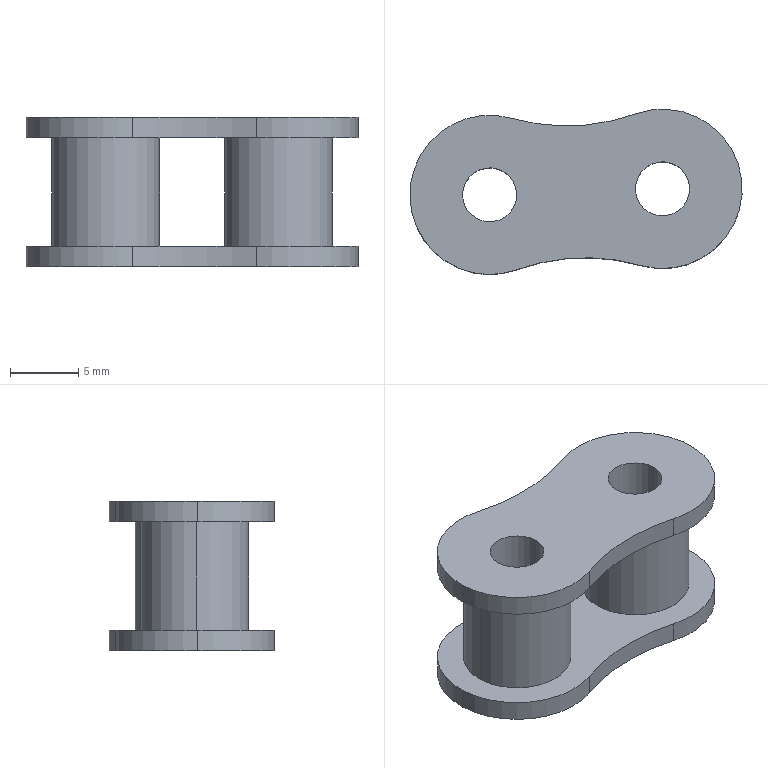Part | STEP file | CHES40-46-Part-17 | 1 solid | 22 faces | box 24.392 x 12.143 x 10.95 mm | volume 1237 mm3 | cylinder 18 | plane 4 | commonest cylinder face diameters 11.7 x6 3.97 x4 7.92 x4 29.64 x4
STEP:
#1=CARTESIAN_POINT('',(-99.678,72.735,-5.475));
#2=VERTEX_POINT('',#1);
#3=CARTESIAN_POINT('',(-103.646,72.597,-5.475));
#4=VERTEX_POINT('',#3);
#5=CARTESIAN_POINT('',(-101.662,72.666,-5.475));
#6=DIRECTION('',(0.,0.,1.));
#7=DIRECTION('',(-0.9994,-0.0349,0.));
#8=AXIS2_PLACEMENT_3D('',#5,#6,#7);
#9=CIRCLE('',#8,1.985);
#10=EDGE_CURVE('',#2,#4,#9,.T.);
#11=ORIENTED_EDGE('',*,*,#10,.F.);
#12=CARTESIAN_POINT('',(-99.678,72.735,5.475));
#13=VERTEX_POINT('',#12);
#14=CARTESIAN_POINT('',(-99.678,72.735,-5.475));
#15=DIRECTION('',(0.,0.,1.));
#16=VECTOR('',#15,1000.);
#17=LINE('',#14,#16);
#18=EDGE_CURVE('',#2,#13,#17,.T.);
#19=ORIENTED_EDGE('',*,*,#18,.T.);
#20=CARTESIAN_POINT('',(-103.646,72.597,5.475));
#21=VERTEX_POINT('',#20);
#22=CARTESIAN_POINT('',(-101.662,72.666,5.475));
#23=DIRECTION('',(0.,0.,1.));
#24=DIRECTION('',(-0.9994,-0.0349,0.));
#25=AXIS2_PLACEMENT_3D('',#22,#23,#24);
#26=CIRCLE('',#25,1.985);
#27=EDGE_CURVE('',#13,#21,#26,.T.);
#28=ORIENTED_EDGE('',*,*,#27,.T.);
#29=CARTESIAN_POINT('',(-103.646,72.597,-5.475));
#30=DIRECTION('',(0.,0.,1.));
#31=VECTOR('',#30,1000.);
#32=LINE('',#29,#31);
#33=EDGE_CURVE('',#4,#21,#32,.T.);
#34=ORIENTED_EDGE('',*,*,#33,.F.);
#35=EDGE_LOOP('',(#11,#19,#28,#34));
#36=FACE_OUTER_BOUND('',#35,.T.);
#37=CARTESIAN_POINT('',(-101.662,72.666,-5.475));
#38=DIRECTION('',(0.,0.,1.));
#39=DIRECTION('',(-0.9994,-0.0349,0.));
#40=AXIS2_PLACEMENT_3D('',#37,#38,#39);
#41=CYLINDRICAL_SURFACE('',#40,1.985);
#42=ADVANCED_FACE('',(#36),#41,.F.);
#43=CARTESIAN_POINT('',(-112.37,72.292,-5.475));
#44=VERTEX_POINT('',#43);
#45=CARTESIAN_POINT('',(-116.338,72.153,-5.475));
#46=VERTEX_POINT('',#45);
#47=CARTESIAN_POINT('',(-114.354,72.223,-5.475));
#48=DIRECTION('',(0.,0.,1.));
#49=DIRECTION('',(-0.9994,-0.0349,0.));
#50=AXIS2_PLACEMENT_3D('',#47,#48,#49);
#51=CIRCLE('',#50,1.985);
#52=EDGE_CURVE('',#44,#46,#51,.T.);
#53=ORIENTED_EDGE('',*,*,#52,.F.);
#54=CARTESIAN_POINT('',(-112.37,72.292,5.475));
#55=VERTEX_POINT('',#54);
#56=CARTESIAN_POINT('',(-112.37,72.292,-5.475));
#57=DIRECTION('',(0.,0.,1.));
#58=VECTOR('',#57,1000.);
#59=LINE('',#56,#58);
#60=EDGE_CURVE('',#44,#55,#59,.T.);
#61=ORIENTED_EDGE('',*,*,#60,.T.);
#62=CARTESIAN_POINT('',(-116.338,72.153,5.475));
#63=VERTEX_POINT('',#62);
#64=CARTESIAN_POINT('',(-114.354,72.223,5.475));
#65=DIRECTION('',(0.,0.,1.));
#66=DIRECTION('',(-0.9994,-0.0349,0.));
#67=AXIS2_PLACEMENT_3D('',#64,#65,#66);
#68=CIRCLE('',#67,1.985);
#69=EDGE_CURVE('',#55,#63,#68,.T.);
#70=ORIENTED_EDGE('',*,*,#69,.T.);
#71=CARTESIAN_POINT('',(-116.338,72.153,-5.475));
#72=DIRECTION('',(0.,0.,1.));
#73=VECTOR('',#72,1000.);
#74=LINE('',#71,#73);
#75=EDGE_CURVE('',#46,#63,#74,.T.);
#76=ORIENTED_EDGE('',*,*,#75,.F.);
#77=EDGE_LOOP('',(#53,#61,#70,#76));
#78=FACE_OUTER_BOUND('',#77,.T.);
#79=CARTESIAN_POINT('',(-114.354,72.223,-5.475));
#80=DIRECTION('',(0.,0.,1.));
#81=DIRECTION('',(-0.9994,-0.0349,0.));
#82=AXIS2_PLACEMENT_3D('',#79,#80,#81);
#83=CYLINDRICAL_SURFACE('',#82,1.985);
#84=ADVANCED_FACE('',(#78),#83,.F.);
#85=CARTESIAN_POINT('',(-120.201,72.018,-5.475));
#86=VERTEX_POINT('',#85);
#87=CARTESIAN_POINT('',(-112.752,77.849,-5.475));
#88=VERTEX_POINT('',#87);
#89=CARTESIAN_POINT('',(-114.354,72.223,-5.475));
#90=DIRECTION('',(0.,0.,-1.));
#91=DIRECTION('',(0.9994,0.0349,0.));
#92=AXIS2_PLACEMENT_3D('',#89,#90,#91);
#93=CIRCLE('',#92,5.85);
#94=EDGE_CURVE('',#86,#88,#93,.T.);
#95=ORIENTED_EDGE('',*,*,#94,.F.);
#96=CARTESIAN_POINT('',(-120.201,72.018,-3.975));
#97=VERTEX_POINT('',#96);
#98=CARTESIAN_POINT('',(-120.201,72.018,-5.475));
#99=DIRECTION('',(0.,0.,1.));
#100=VECTOR('',#99,1000.);
#101=LINE('',#98,#100);
#102=EDGE_CURVE('',#86,#97,#101,.T.);
#103=ORIENTED_EDGE('',*,*,#102,.T.);
#104=CARTESIAN_POINT('',(-112.752,77.849,-3.975));
#105=VERTEX_POINT('',#104);
#106=CARTESIAN_POINT('',(-114.354,72.223,-3.975));
#107=DIRECTION('',(0.,0.,-1.));
#108=DIRECTION('',(0.9994,0.0349,0.));
#109=AXIS2_PLACEMENT_3D('',#106,#107,#108);
#110=CIRCLE('',#109,5.85);
#111=EDGE_CURVE('',#97,#105,#110,.T.);
#112=ORIENTED_EDGE('',*,*,#111,.T.);
#113=CARTESIAN_POINT('',(-112.752,77.849,-5.475));
#114=DIRECTION('',(0.,0.,1.));
#115=VECTOR('',#114,1000.);
#116=LINE('',#113,#115);
#117=EDGE_CURVE('',#88,#105,#116,.T.);
#118=ORIENTED_EDGE('',*,*,#117,.F.);
#119=EDGE_LOOP('',(#95,#103,#112,#118));
#120=FACE_OUTER_BOUND('',#119,.T.);
#121=CARTESIAN_POINT('',(-114.354,72.223,-5.475));
#122=DIRECTION('',(0.,0.,1.));
#123=DIRECTION('',(-0.9994,-0.0349,0.));
#124=AXIS2_PLACEMENT_3D('',#121,#122,#123);
#125=CYLINDRICAL_SURFACE('',#124,5.85);
#126=ADVANCED_FACE('',(#120),#125,.T.);
#127=CARTESIAN_POINT('',(-110.397,72.361,3.975));
#128=VERTEX_POINT('',#127);
#129=CARTESIAN_POINT('',(-118.312,72.084,3.975));
#130=VERTEX_POINT('',#129);
#131=CARTESIAN_POINT('',(-114.354,72.223,3.975));
#132=DIRECTION('',(0.,0.,-1.));
#133=DIRECTION('',(-0.9994,-0.0349,0.));
#134=AXIS2_PLACEMENT_3D('',#131,#132,#133);
#135=CIRCLE('',#134,3.96);
#136=EDGE_CURVE('',#128,#130,#135,.T.);
#137=ORIENTED_EDGE('',*,*,#136,.T.);
#138=CARTESIAN_POINT('',(-118.312,72.084,-3.975));
#139=VERTEX_POINT('',#138);
#140=CARTESIAN_POINT('',(-118.312,72.084,-3.975));
#141=DIRECTION('',(0.,0.,-1.));
#142=VECTOR('',#141,1000.);
#143=LINE('',#140,#142);
#144=EDGE_CURVE('',#130,#139,#143,.T.);
#145=ORIENTED_EDGE('',*,*,#144,.T.);
#146=CARTESIAN_POINT('',(-110.397,72.361,-3.975));
#147=VERTEX_POINT('',#146);
#148=CARTESIAN_POINT('',(-114.354,72.223,-3.975));
#149=DIRECTION('',(0.,0.,-1.));
#150=DIRECTION('',(0.9994,0.0349,0.));
#151=AXIS2_PLACEMENT_3D('',#148,#149,#150);
#152=CIRCLE('',#151,3.96);
#153=EDGE_CURVE('',#147,#139,#152,.T.);
#154=ORIENTED_EDGE('',*,*,#153,.F.);
#155=CARTESIAN_POINT('',(-110.397,72.361,-3.975));
#156=DIRECTION('',(0.,0.,-1.));
#157=VECTOR('',#156,1000.);
#158=LINE('',#155,#157);
#159=EDGE_CURVE('',#128,#147,#158,.T.);
#160=ORIENTED_EDGE('',*,*,#159,.F.);
#161=EDGE_LOOP('',(#137,#145,#154,#160));
#162=FACE_OUTER_BOUND('',#161,.T.);
#163=CARTESIAN_POINT('',(-114.354,72.223,-3.975));
#164=DIRECTION('',(0.,0.,-1.));
#165=DIRECTION('',(0.9994,0.0349,0.));
#166=AXIS2_PLACEMENT_3D('',#163,#164,#165);
#167=CYLINDRICAL_SURFACE('',#166,3.96);
#168=ADVANCED_FACE('',(#162),#167,.T.);
#169=CARTESIAN_POINT('',(-112.364,66.722,5.475));
#170=VERTEX_POINT('',#169);
#171=CARTESIAN_POINT('',(-120.201,72.018,5.475));
#172=VERTEX_POINT('',#171);
#173=CARTESIAN_POINT('',(-114.354,72.223,5.475));
#174=DIRECTION('',(0.,0.,-1.));
#175=DIRECTION('',(0.9994,0.0349,0.));
#176=AXIS2_PLACEMENT_3D('',#173,#174,#175);
#177=CIRCLE('',#176,5.85);
#178=EDGE_CURVE('',#170,#172,#177,.T.);
#179=ORIENTED_EDGE('',*,*,#178,.T.);
#180=CARTESIAN_POINT('',(-120.201,72.018,3.975));
#181=VERTEX_POINT('',#180);
#182=CARTESIAN_POINT('',(-120.201,72.018,5.475));
#183=DIRECTION('',(0.,0.,-1.));
#184=VECTOR('',#183,1000.);
#185=LINE('',#182,#184);
#186=EDGE_CURVE('',#172,#181,#185,.T.);
#187=ORIENTED_EDGE('',*,*,#186,.T.);
#188=CARTESIAN_POINT('',(-112.364,66.722,3.975));
#189=VERTEX_POINT('',#188);
#190=CARTESIAN_POINT('',(-114.354,72.223,3.975));
#191=DIRECTION('',(0.,0.,-1.));
#192=DIRECTION('',(0.9994,0.0349,0.));
#193=AXIS2_PLACEMENT_3D('',#190,#191,#192);
#194=CIRCLE('',#193,5.85);
#195=EDGE_CURVE('',#189,#181,#194,.T.);
#196=ORIENTED_EDGE('',*,*,#195,.F.);
#197=CARTESIAN_POINT('',(-112.364,66.722,5.475));
#198=DIRECTION('',(0.,0.,-1.));
#199=VECTOR('',#198,1000.);
#200=LINE('',#197,#199);
#201=EDGE_CURVE('',#170,#189,#200,.T.);
#202=ORIENTED_EDGE('',*,*,#201,.F.);
#203=EDGE_LOOP('',(#179,#187,#196,#202));
#204=FACE_OUTER_BOUND('',#203,.T.);
#205=CARTESIAN_POINT('',(-114.354,72.223,5.475));
#206=DIRECTION('',(0.,0.,-1.));
#207=DIRECTION('',(-0.9994,-0.0349,0.));
#208=AXIS2_PLACEMENT_3D('',#205,#206,#207);
#209=CYLINDRICAL_SURFACE('',#208,5.85);
#210=ADVANCED_FACE('',(#204),#209,.T.);
#211=CARTESIAN_POINT('',(-105.619,72.528,3.975));
#212=VERTEX_POINT('',#211);
#213=CARTESIAN_POINT('',(-97.704,72.804,3.975));
#214=VERTEX_POINT('',#213);
#215=CARTESIAN_POINT('',(-101.662,72.666,3.975));
#216=DIRECTION('',(0.,0.,1.));
#217=DIRECTION('',(-0.9994,-0.0349,0.));
#218=AXIS2_PLACEMENT_3D('',#215,#216,#217);
#219=CIRCLE('',#218,3.96);
#220=EDGE_CURVE('',#212,#214,#219,.T.);
#221=ORIENTED_EDGE('',*,*,#220,.F.);
#222=CARTESIAN_POINT('',(-105.619,72.528,-3.975));
#223=VERTEX_POINT('',#222);
#224=CARTESIAN_POINT('',(-105.619,72.528,-3.975));
#225=DIRECTION('',(0.,0.,-1.));
#226=VECTOR('',#225,1000.);
#227=LINE('',#224,#226);
#228=EDGE_CURVE('',#212,#223,#227,.T.);
#229=ORIENTED_EDGE('',*,*,#228,.T.);
#230=CARTESIAN_POINT('',(-97.704,72.804,-3.975));
#231=VERTEX_POINT('',#230);
#232=CARTESIAN_POINT('',(-101.662,72.666,-3.975));
#233=DIRECTION('',(0.,0.,-1.));
#234=DIRECTION('',(0.9994,0.0349,0.));
#235=AXIS2_PLACEMENT_3D('',#232,#233,#234);
#236=CIRCLE('',#235,3.96);
#237=EDGE_CURVE('',#231,#223,#236,.T.);
#238=ORIENTED_EDGE('',*,*,#237,.F.);
#239=CARTESIAN_POINT('',(-97.704,72.804,-3.975));
#240=DIRECTION('',(0.,0.,-1.));
#241=VECTOR('',#240,1000.);
#242=LINE('',#239,#241);
#243=EDGE_CURVE('',#214,#231,#242,.T.);
#244=ORIENTED_EDGE('',*,*,#243,.F.);
#245=EDGE_LOOP('',(#221,#229,#238,#244));
#246=FACE_OUTER_BOUND('',#245,.T.);
#247=CARTESIAN_POINT('',(-101.662,72.666,-3.975));
#248=DIRECTION('',(0.,0.,-1.));
#249=DIRECTION('',(0.9994,0.0349,0.));
#250=AXIS2_PLACEMENT_3D('',#247,#248,#249);
#251=CYLINDRICAL_SURFACE('',#250,3.96);
#252=ADVANCED_FACE('',(#246),#251,.T.);
#253=ORIENTED_EDGE('',*,*,#195,.T.);
#254=CARTESIAN_POINT('',(-112.752,77.849,3.975));
#255=VERTEX_POINT('',#254);
#256=CARTESIAN_POINT('',(-114.354,72.223,3.975));
#257=DIRECTION('',(0.,0.,-1.));
#258=DIRECTION('',(0.9994,0.0349,0.));
#259=AXIS2_PLACEMENT_3D('',#256,#257,#258);
#260=CIRCLE('',#259,5.85);
#261=EDGE_CURVE('',#181,#255,#260,.T.);
#262=ORIENTED_EDGE('',*,*,#261,.T.);
#263=CARTESIAN_POINT('',(-103.652,78.167,3.975));
#264=VERTEX_POINT('',#263);
#265=CARTESIAN_POINT('',(-108.695,92.103,3.975));
#266=DIRECTION('',(0.,0.,1.));
#267=DIRECTION('',(-0.9994,-0.0349,0.));
#268=AXIS2_PLACEMENT_3D('',#265,#266,#267);
#269=CIRCLE('',#268,14.82);
#270=EDGE_CURVE('',#255,#264,#269,.T.);
#271=ORIENTED_EDGE('',*,*,#270,.T.);
#272=CARTESIAN_POINT('',(-103.264,67.039,3.975));
#273=VERTEX_POINT('',#272);
#274=CARTESIAN_POINT('',(-101.662,72.666,3.975));
#275=DIRECTION('',(0.,0.,-1.));
#276=DIRECTION('',(-0.9994,-0.0349,0.));
#277=AXIS2_PLACEMENT_3D('',#274,#275,#276);
#278=CIRCLE('',#277,5.85);
#279=EDGE_CURVE('',#264,#273,#278,.T.);
#280=ORIENTED_EDGE('',*,*,#279,.T.);
#281=CARTESIAN_POINT('',(-107.322,52.786,3.975));
#282=DIRECTION('',(0.,0.,1.));
#283=DIRECTION('',(0.9994,0.0349,0.));
#284=AXIS2_PLACEMENT_3D('',#281,#282,#283);
#285=CIRCLE('',#284,14.82);
#286=EDGE_CURVE('',#273,#189,#285,.T.);
#287=ORIENTED_EDGE('',*,*,#286,.T.);
#288=EDGE_LOOP('',(#253,#262,#271,#280,#287));
#289=FACE_OUTER_BOUND('',#288,.T.);
#290=CARTESIAN_POINT('',(-101.662,72.666,3.975));
#291=DIRECTION('',(0.,0.,1.));
#292=DIRECTION('',(-0.9994,-0.0349,0.));
#293=AXIS2_PLACEMENT_3D('',#290,#291,#292);
#294=CIRCLE('',#293,3.96);
#295=EDGE_CURVE('',#214,#212,#294,.T.);
#296=ORIENTED_EDGE('',*,*,#295,.T.);
#297=ORIENTED_EDGE('',*,*,#220,.T.);
#298=EDGE_LOOP('',(#296,#297));
#299=FACE_BOUND('',#298,.T.);
#300=ORIENTED_EDGE('',*,*,#136,.F.);
#301=CARTESIAN_POINT('',(-114.354,72.223,3.975));
#302=DIRECTION('',(0.,0.,-1.));
#303=DIRECTION('',(-0.9994,-0.0349,0.));
#304=AXIS2_PLACEMENT_3D('',#301,#302,#303);
#305=CIRCLE('',#304,3.96);
#306=EDGE_CURVE('',#130,#128,#305,.T.);
#307=ORIENTED_EDGE('',*,*,#306,.F.);
#308=EDGE_LOOP('',(#300,#307));
#309=FACE_BOUND('',#308,.T.);
#310=CARTESIAN_POINT('',(-111.524,82.163,3.975));
#311=DIRECTION('',(0.,0.,1.));
#312=DIRECTION('',(0.9994,0.0349,0.));
#313=AXIS2_PLACEMENT_3D('',#310,#311,#312);
#314=PLANE('',#313);
#315=ADVANCED_FACE('',(#289,#299,#309),#314,.F.);
#316=ORIENTED_EDGE('',*,*,#228,.F.);
#317=ORIENTED_EDGE('',*,*,#295,.F.);
#318=ORIENTED_EDGE('',*,*,#243,.T.);
#319=CARTESIAN_POINT('',(-101.662,72.666,-3.975));
#320=DIRECTION('',(0.,0.,-1.));
#321=DIRECTION('',(0.9994,0.0349,0.));
#322=AXIS2_PLACEMENT_3D('',#319,#320,#321);
#323=CIRCLE('',#322,3.96);
#324=EDGE_CURVE('',#223,#231,#323,.T.);
#325=ORIENTED_EDGE('',*,*,#324,.F.);
#326=EDGE_LOOP('',(#316,#317,#318,#325));
#327=FACE_OUTER_BOUND('',#326,.T.);
#328=CARTESIAN_POINT('',(-101.662,72.666,-3.975));
#329=DIRECTION('',(0.,0.,-1.));
#330=DIRECTION('',(0.9994,0.0349,0.));
#331=AXIS2_PLACEMENT_3D('',#328,#329,#330);
#332=CYLINDRICAL_SURFACE('',#331,3.96);
#333=ADVANCED_FACE('',(#327),#332,.T.);
#334=ORIENTED_EDGE('',*,*,#186,.F.);
#335=CARTESIAN_POINT('',(-112.752,77.849,5.475));
#336=VERTEX_POINT('',#335);
#337=CARTESIAN_POINT('',(-114.354,72.223,5.475));
#338=DIRECTION('',(0.,0.,-1.));
#339=DIRECTION('',(0.9994,0.0349,0.));
#340=AXIS2_PLACEMENT_3D('',#337,#338,#339);
#341=CIRCLE('',#340,5.85);
#342=EDGE_CURVE('',#172,#336,#341,.T.);
#343=ORIENTED_EDGE('',*,*,#342,.T.);
#344=CARTESIAN_POINT('',(-112.752,77.849,5.475));
#345=DIRECTION('',(0.,0.,-1.));
#346=VECTOR('',#345,1000.);
#347=LINE('',#344,#346);
#348=EDGE_CURVE('',#336,#255,#347,.T.);
#349=ORIENTED_EDGE('',*,*,#348,.T.);
#350=ORIENTED_EDGE('',*,*,#261,.F.);
#351=EDGE_LOOP('',(#334,#343,#349,#350));
#352=FACE_OUTER_BOUND('',#351,.T.);
#353=CARTESIAN_POINT('',(-114.354,72.223,5.475));
#354=DIRECTION('',(0.,0.,-1.));
#355=DIRECTION('',(-0.9994,-0.0349,0.));
#356=AXIS2_PLACEMENT_3D('',#353,#354,#355);
#357=CYLINDRICAL_SURFACE('',#356,5.85);
#358=ADVANCED_FACE('',(#352),#357,.T.);
#359=ORIENTED_EDGE('',*,*,#270,.F.);
#360=ORIENTED_EDGE('',*,*,#348,.F.);
#361=CARTESIAN_POINT('',(-103.652,78.167,5.475));
#362=VERTEX_POINT('',#361);
#363=CARTESIAN_POINT('',(-108.695,92.103,5.475));
#364=DIRECTION('',(0.,0.,1.));
#365=DIRECTION('',(-0.9994,-0.0349,0.));
#366=AXIS2_PLACEMENT_3D('',#363,#364,#365);
#367=CIRCLE('',#366,14.82);
#368=EDGE_CURVE('',#336,#362,#367,.T.);
#369=ORIENTED_EDGE('',*,*,#368,.T.);
#370=CARTESIAN_POINT('',(-103.652,78.167,5.475));
#371=DIRECTION('',(0.,0.,-1.));
#372=VECTOR('',#371,1000.);
#373=LINE('',#370,#372);
#374=EDGE_CURVE('',#362,#264,#373,.T.);
#375=ORIENTED_EDGE('',*,*,#374,.T.);
#376=EDGE_LOOP('',(#359,#360,#369,#375));
#377=FACE_OUTER_BOUND('',#376,.T.);
#378=CARTESIAN_POINT('',(-108.695,92.103,5.475));
#379=DIRECTION('',(0.,0.,-1.));
#380=DIRECTION('',(-0.9994,-0.0349,0.));
#381=AXIS2_PLACEMENT_3D('',#378,#379,#380);
#382=CYLINDRICAL_SURFACE('',#381,14.82);
#383=ADVANCED_FACE('',(#377),#382,.F.);
#384=ORIENTED_EDGE('',*,*,#279,.F.);
#385=ORIENTED_EDGE('',*,*,#374,.F.);
#386=CARTESIAN_POINT('',(-103.264,67.039,5.475));
#387=VERTEX_POINT('',#386);
#388=CARTESIAN_POINT('',(-101.662,72.666,5.475));
#389=DIRECTION('',(0.,0.,-1.));
#390=DIRECTION('',(-0.9994,-0.0349,0.));
#391=AXIS2_PLACEMENT_3D('',#388,#389,#390);
#392=CIRCLE('',#391,5.85);
#393=EDGE_CURVE('',#362,#387,#392,.T.);
#394=ORIENTED_EDGE('',*,*,#393,.T.);
#395=CARTESIAN_POINT('',(-103.264,67.039,5.475));
#396=DIRECTION('',(0.,0.,-1.));
#397=VECTOR('',#396,1000.);
#398=LINE('',#395,#397);
#399=EDGE_CURVE('',#387,#273,#398,.T.);
#400=ORIENTED_EDGE('',*,*,#399,.T.);
#401=EDGE_LOOP('',(#384,#385,#394,#400));
#402=FACE_OUTER_BOUND('',#401,.T.);
#403=CARTESIAN_POINT('',(-101.662,72.666,5.475));
#404=DIRECTION('',(0.,0.,-1.));
#405=DIRECTION('',(-0.9994,-0.0349,0.));
#406=AXIS2_PLACEMENT_3D('',#403,#404,#405);
#407=CYLINDRICAL_SURFACE('',#406,5.85);
#408=ADVANCED_FACE('',(#402),#407,.T.);
#409=ORIENTED_EDGE('',*,*,#286,.F.);
#410=ORIENTED_EDGE('',*,*,#399,.F.);
#411=CARTESIAN_POINT('',(-107.322,52.786,5.475));
#412=DIRECTION('',(0.,0.,1.));
#413=DIRECTION('',(0.9994,0.0349,0.));
#414=AXIS2_PLACEMENT_3D('',#411,#412,#413);
#415=CIRCLE('',#414,14.82);
#416=EDGE_CURVE('',#387,#170,#415,.T.);
#417=ORIENTED_EDGE('',*,*,#416,.T.);
#418=ORIENTED_EDGE('',*,*,#201,.T.);
#419=EDGE_LOOP('',(#409,#410,#417,#418));
#420=FACE_OUTER_BOUND('',#419,.T.);
#421=CARTESIAN_POINT('',(-107.322,52.786,5.475));
#422=DIRECTION('',(0.,0.,-1.));
#423=DIRECTION('',(-0.9994,-0.0349,0.));
#424=AXIS2_PLACEMENT_3D('',#421,#422,#423);
#425=CYLINDRICAL_SURFACE('',#424,14.82);
#426=ADVANCED_FACE('',(#420),#425,.F.);
#427=CARTESIAN_POINT('',(-101.662,72.666,5.475));
#428=DIRECTION('',(0.,0.,1.));
#429=DIRECTION('',(-0.9994,-0.0349,0.));
#430=AXIS2_PLACEMENT_3D('',#427,#428,#429);
#431=CIRCLE('',#430,1.985);
#432=EDGE_CURVE('',#21,#13,#431,.T.);
#433=ORIENTED_EDGE('',*,*,#432,.F.);
#434=ORIENTED_EDGE('',*,*,#27,.F.);
#435=EDGE_LOOP('',(#433,#434));
#436=FACE_BOUND('',#435,.T.);
#437=CARTESIAN_POINT('',(-114.354,72.223,5.475));
#438=DIRECTION('',(0.,0.,1.));
#439=DIRECTION('',(-0.9994,-0.0349,0.));
#440=AXIS2_PLACEMENT_3D('',#437,#438,#439);
#441=CIRCLE('',#440,1.985);
#442=EDGE_CURVE('',#63,#55,#441,.T.);
#443=ORIENTED_EDGE('',*,*,#442,.F.);
#444=ORIENTED_EDGE('',*,*,#69,.F.);
#445=EDGE_LOOP('',(#443,#444));
#446=FACE_BOUND('',#445,.T.);
#447=ORIENTED_EDGE('',*,*,#178,.F.);
#448=ORIENTED_EDGE('',*,*,#416,.F.);
#449=ORIENTED_EDGE('',*,*,#393,.F.);
#450=ORIENTED_EDGE('',*,*,#368,.F.);
#451=ORIENTED_EDGE('',*,*,#342,.F.);
#452=EDGE_LOOP('',(#447,#448,#449,#450,#451));
#453=FACE_OUTER_BOUND('',#452,.T.);
#454=CARTESIAN_POINT('',(-111.524,82.163,5.475));
#455=DIRECTION('',(0.,0.,1.));
#456=DIRECTION('',(0.9994,0.0349,0.));
#457=AXIS2_PLACEMENT_3D('',#454,#455,#456);
#458=PLANE('',#457);
#459=ADVANCED_FACE('',(#436,#446,#453),#458,.T.);
#460=ORIENTED_EDGE('',*,*,#144,.F.);
#461=ORIENTED_EDGE('',*,*,#306,.T.);
#462=ORIENTED_EDGE('',*,*,#159,.T.);
#463=CARTESIAN_POINT('',(-114.354,72.223,-3.975));
#464=DIRECTION('',(0.,0.,-1.));
#465=DIRECTION('',(0.9994,0.0349,0.));
#466=AXIS2_PLACEMENT_3D('',#463,#464,#465);
#467=CIRCLE('',#466,3.96);
#468=EDGE_CURVE('',#139,#147,#467,.T.);
#469=ORIENTED_EDGE('',*,*,#468,.F.);
#470=EDGE_LOOP('',(#460,#461,#462,#469));
#471=FACE_OUTER_BOUND('',#470,.T.);
#472=CARTESIAN_POINT('',(-114.354,72.223,-3.975));
#473=DIRECTION('',(0.,0.,-1.));
#474=DIRECTION('',(0.9994,0.0349,0.));
#475=AXIS2_PLACEMENT_3D('',#472,#473,#474);
#476=CYLINDRICAL_SURFACE('',#475,3.96);
#477=ADVANCED_FACE('',(#471),#476,.T.);
#478=ORIENTED_EDGE('',*,*,#153,.T.);
#479=ORIENTED_EDGE('',*,*,#468,.T.);
#480=EDGE_LOOP('',(#478,#479));
#481=FACE_BOUND('',#480,.T.);
#482=CARTESIAN_POINT('',(-112.364,66.722,-3.975));
#483=VERTEX_POINT('',#482);
#484=CARTESIAN_POINT('',(-114.354,72.223,-3.975));
#485=DIRECTION('',(0.,0.,-1.));
#486=DIRECTION('',(0.9994,0.0349,0.));
#487=AXIS2_PLACEMENT_3D('',#484,#485,#486);
#488=CIRCLE('',#487,5.85);
#489=EDGE_CURVE('',#483,#97,#488,.T.);
#490=ORIENTED_EDGE('',*,*,#489,.F.);
#491=CARTESIAN_POINT('',(-103.264,67.039,-3.975));
#492=VERTEX_POINT('',#491);
#493=CARTESIAN_POINT('',(-107.322,52.786,-3.975));
#494=DIRECTION('',(0.,0.,1.));
#495=DIRECTION('',(0.9994,0.0349,0.));
#496=AXIS2_PLACEMENT_3D('',#493,#494,#495);
#497=CIRCLE('',#496,14.82);
#498=EDGE_CURVE('',#492,#483,#497,.T.);
#499=ORIENTED_EDGE('',*,*,#498,.F.);
#500=CARTESIAN_POINT('',(-103.652,78.167,-3.975));
#501=VERTEX_POINT('',#500);
#502=CARTESIAN_POINT('',(-101.662,72.666,-3.975));
#503=DIRECTION('',(0.,0.,-1.));
#504=DIRECTION('',(-0.9994,-0.0349,0.));
#505=AXIS2_PLACEMENT_3D('',#502,#503,#504);
#506=CIRCLE('',#505,5.85);
#507=EDGE_CURVE('',#501,#492,#506,.T.);
#508=ORIENTED_EDGE('',*,*,#507,.F.);
#509=CARTESIAN_POINT('',(-108.695,92.103,-3.975));
#510=DIRECTION('',(0.,0.,1.));
#511=DIRECTION('',(-0.9994,-0.0349,0.));
#512=AXIS2_PLACEMENT_3D('',#509,#510,#511);
#513=CIRCLE('',#512,14.82);
#514=EDGE_CURVE('',#105,#501,#513,.T.);
#515=ORIENTED_EDGE('',*,*,#514,.F.);
#516=ORIENTED_EDGE('',*,*,#111,.F.);
#517=EDGE_LOOP('',(#490,#499,#508,#515,#516));
#518=FACE_OUTER_BOUND('',#517,.T.);
#519=ORIENTED_EDGE('',*,*,#237,.T.);
#520=ORIENTED_EDGE('',*,*,#324,.T.);
#521=EDGE_LOOP('',(#519,#520));
#522=FACE_BOUND('',#521,.T.);
#523=CARTESIAN_POINT('',(-111.524,82.163,-3.975));
#524=DIRECTION('',(0.,0.,-1.));
#525=DIRECTION('',(0.9994,0.0349,0.));
#526=AXIS2_PLACEMENT_3D('',#523,#524,#525);
#527=PLANE('',#526);
#528=ADVANCED_FACE('',(#481,#518,#522),#527,.F.);
#529=ORIENTED_EDGE('',*,*,#102,.F.);
#530=CARTESIAN_POINT('',(-112.364,66.722,-5.475));
#531=VERTEX_POINT('',#530);
#532=CARTESIAN_POINT('',(-114.354,72.223,-5.475));
#533=DIRECTION('',(0.,0.,-1.));
#534=DIRECTION('',(0.9994,0.0349,0.));
#535=AXIS2_PLACEMENT_3D('',#532,#533,#534);
#536=CIRCLE('',#535,5.85);
#537=EDGE_CURVE('',#531,#86,#536,.T.);
#538=ORIENTED_EDGE('',*,*,#537,.F.);
#539=CARTESIAN_POINT('',(-112.364,66.722,-5.475));
#540=DIRECTION('',(0.,0.,1.));
#541=VECTOR('',#540,1000.);
#542=LINE('',#539,#541);
#543=EDGE_CURVE('',#531,#483,#542,.T.);
#544=ORIENTED_EDGE('',*,*,#543,.T.);
#545=ORIENTED_EDGE('',*,*,#489,.T.);
#546=EDGE_LOOP('',(#529,#538,#544,#545));
#547=FACE_OUTER_BOUND('',#546,.T.);
#548=CARTESIAN_POINT('',(-114.354,72.223,-5.475));
#549=DIRECTION('',(0.,0.,1.));
#550=DIRECTION('',(-0.9994,-0.0349,0.));
#551=AXIS2_PLACEMENT_3D('',#548,#549,#550);
#552=CYLINDRICAL_SURFACE('',#551,5.85);
#553=ADVANCED_FACE('',(#547),#552,.T.);
#554=ORIENTED_EDGE('',*,*,#514,.T.);
#555=CARTESIAN_POINT('',(-103.652,78.167,-5.475));
#556=VERTEX_POINT('',#555);
#557=CARTESIAN_POINT('',(-103.652,78.167,-5.475));
#558=DIRECTION('',(0.,0.,1.));
#559=VECTOR('',#558,1000.);
#560=LINE('',#557,#559);
#561=EDGE_CURVE('',#556,#501,#560,.T.);
#562=ORIENTED_EDGE('',*,*,#561,.F.);
#563=CARTESIAN_POINT('',(-108.695,92.103,-5.475));
#564=DIRECTION('',(0.,0.,1.));
#565=DIRECTION('',(-0.9994,-0.0349,0.));
#566=AXIS2_PLACEMENT_3D('',#563,#564,#565);
#567=CIRCLE('',#566,14.82);
#568=EDGE_CURVE('',#88,#556,#567,.T.);
#569=ORIENTED_EDGE('',*,*,#568,.F.);
#570=ORIENTED_EDGE('',*,*,#117,.T.);
#571=EDGE_LOOP('',(#554,#562,#569,#570));
#572=FACE_OUTER_BOUND('',#571,.T.);
#573=CARTESIAN_POINT('',(-108.695,92.103,-5.475));
#574=DIRECTION('',(0.,0.,1.));
#575=DIRECTION('',(-0.9994,-0.0349,0.));
#576=AXIS2_PLACEMENT_3D('',#573,#574,#575);
#577=CYLINDRICAL_SURFACE('',#576,14.82);
#578=ADVANCED_FACE('',(#572),#577,.F.);
#579=ORIENTED_EDGE('',*,*,#507,.T.);
#580=CARTESIAN_POINT('',(-103.264,67.039,-5.475));
#581=VERTEX_POINT('',#580);
#582=CARTESIAN_POINT('',(-103.264,67.039,-5.475));
#583=DIRECTION('',(0.,0.,1.));
#584=VECTOR('',#583,1000.);
#585=LINE('',#582,#584);
#586=EDGE_CURVE('',#581,#492,#585,.T.);
#587=ORIENTED_EDGE('',*,*,#586,.F.);
#588=CARTESIAN_POINT('',(-101.662,72.666,-5.475));
#589=DIRECTION('',(0.,0.,-1.));
#590=DIRECTION('',(-0.9994,-0.0349,0.));
#591=AXIS2_PLACEMENT_3D('',#588,#589,#590);
#592=CIRCLE('',#591,5.85);
#593=EDGE_CURVE('',#556,#581,#592,.T.);
#594=ORIENTED_EDGE('',*,*,#593,.F.);
#595=ORIENTED_EDGE('',*,*,#561,.T.);
#596=EDGE_LOOP('',(#579,#587,#594,#595));
#597=FACE_OUTER_BOUND('',#596,.T.);
#598=CARTESIAN_POINT('',(-101.662,72.666,-5.475));
#599=DIRECTION('',(0.,0.,1.));
#600=DIRECTION('',(-0.9994,-0.0349,0.));
#601=AXIS2_PLACEMENT_3D('',#598,#599,#600);
#602=CYLINDRICAL_SURFACE('',#601,5.85);
#603=ADVANCED_FACE('',(#597),#602,.T.);
#604=ORIENTED_EDGE('',*,*,#498,.T.);
#605=ORIENTED_EDGE('',*,*,#543,.F.);
#606=CARTESIAN_POINT('',(-107.322,52.786,-5.475));
#607=DIRECTION('',(0.,0.,1.));
#608=DIRECTION('',(0.9994,0.0349,0.));
#609=AXIS2_PLACEMENT_3D('',#606,#607,#608);
#610=CIRCLE('',#609,14.82);
#611=EDGE_CURVE('',#581,#531,#610,.T.);
#612=ORIENTED_EDGE('',*,*,#611,.F.);
#613=ORIENTED_EDGE('',*,*,#586,.T.);
#614=EDGE_LOOP('',(#604,#605,#612,#613));
#615=FACE_OUTER_BOUND('',#614,.T.);
#616=CARTESIAN_POINT('',(-107.322,52.786,-5.475));
#617=DIRECTION('',(0.,0.,1.));
#618=DIRECTION('',(-0.9994,-0.0349,0.));
#619=AXIS2_PLACEMENT_3D('',#616,#617,#618);
#620=CYLINDRICAL_SURFACE('',#619,14.82);
#621=ADVANCED_FACE('',(#615),#620,.F.);
#622=CARTESIAN_POINT('',(-101.662,72.666,-5.475));
#623=DIRECTION('',(0.,0.,1.));
#624=DIRECTION('',(-0.9994,-0.0349,0.));
#625=AXIS2_PLACEMENT_3D('',#622,#623,#624);
#626=CIRCLE('',#625,1.985);
#627=EDGE_CURVE('',#4,#2,#626,.T.);
#628=ORIENTED_EDGE('',*,*,#627,.T.);
#629=ORIENTED_EDGE('',*,*,#10,.T.);
#630=EDGE_LOOP('',(#628,#629));
#631=FACE_BOUND('',#630,.T.);
#632=CARTESIAN_POINT('',(-114.354,72.223,-5.475));
#633=DIRECTION('',(0.,0.,1.));
#634=DIRECTION('',(-0.9994,-0.0349,0.));
#635=AXIS2_PLACEMENT_3D('',#632,#633,#634);
#636=CIRCLE('',#635,1.985);
#637=EDGE_CURVE('',#46,#44,#636,.T.);
#638=ORIENTED_EDGE('',*,*,#637,.T.);
#639=ORIENTED_EDGE('',*,*,#52,.T.);
#640=EDGE_LOOP('',(#638,#639));
#641=FACE_BOUND('',#640,.T.);
#642=ORIENTED_EDGE('',*,*,#537,.T.);
#643=ORIENTED_EDGE('',*,*,#94,.T.);
#644=ORIENTED_EDGE('',*,*,#568,.T.);
#645=ORIENTED_EDGE('',*,*,#593,.T.);
#646=ORIENTED_EDGE('',*,*,#611,.T.);
#647=EDGE_LOOP('',(#642,#643,#644,#645,#646));
#648=FACE_OUTER_BOUND('',#647,.T.);
#649=CARTESIAN_POINT('',(-111.524,82.163,-5.475));
#650=DIRECTION('',(0.,0.,-1.));
#651=DIRECTION('',(0.9994,0.0349,0.));
#652=AXIS2_PLACEMENT_3D('',#649,#650,#651);
#653=PLANE('',#652);
#654=ADVANCED_FACE('',(#631,#641,#648),#653,.T.);
#655=ORIENTED_EDGE('',*,*,#60,.F.);
#656=ORIENTED_EDGE('',*,*,#637,.F.);
#657=ORIENTED_EDGE('',*,*,#75,.T.);
#658=ORIENTED_EDGE('',*,*,#442,.T.);
#659=EDGE_LOOP('',(#655,#656,#657,#658));
#660=FACE_OUTER_BOUND('',#659,.T.);
#661=CARTESIAN_POINT('',(-114.354,72.223,-5.475));
#662=DIRECTION('',(0.,0.,1.));
#663=DIRECTION('',(-0.9994,-0.0349,0.));
#664=AXIS2_PLACEMENT_3D('',#661,#662,#663);
#665=CYLINDRICAL_SURFACE('',#664,1.985);
#666=ADVANCED_FACE('',(#660),#665,.F.);
#667=ORIENTED_EDGE('',*,*,#18,.F.);
#668=ORIENTED_EDGE('',*,*,#627,.F.);
#669=ORIENTED_EDGE('',*,*,#33,.T.);
#670=ORIENTED_EDGE('',*,*,#432,.T.);
#671=EDGE_LOOP('',(#667,#668,#669,#670));
#672=FACE_OUTER_BOUND('',#671,.T.);
#673=CARTESIAN_POINT('',(-101.662,72.666,-5.475));
#674=DIRECTION('',(0.,0.,1.));
#675=DIRECTION('',(-0.9994,-0.0349,0.));
#676=AXIS2_PLACEMENT_3D('',#673,#674,#675);
#677=CYLINDRICAL_SURFACE('',#676,1.985);
#678=ADVANCED_FACE('',(#672),#677,.F.);
#679=CLOSED_SHELL('',(#42,#84,#126,#168,#210,#252,#315,#333,#358,#383,#408,#426,#459,#477,#528,#553,#578,#603,#621,#654,#666,#678));
#680=MANIFOLD_SOLID_BREP('',#679);
#681=CARTESIAN_POINT('',(0.,0.,0.));
#682=DIRECTION('',(0.,0.,1.));
#683=DIRECTION('',(1.,0.,0.));
#684=AXIS2_PLACEMENT_3D('',#681,#682,#683);
#685=(LENGTH_UNIT()NAMED_UNIT(*)SI_UNIT(.MILLI.,.METRE.));
#686=UNCERTAINTY_MEASURE_WITH_UNIT(LENGTH_MEASURE(0.00001),#685,'','');
#687=(NAMED_UNIT(*)PLANE_ANGLE_UNIT()SI_UNIT($,.RADIAN.));
#688=(NAMED_UNIT(*)SI_UNIT($,.STERADIAN.)SOLID_ANGLE_UNIT());
#689=(GEOMETRIC_REPRESENTATION_CONTEXT(3)GLOBAL_UNCERTAINTY_ASSIGNED_CONTEXT((#686))GLOBAL_UNIT_ASSIGNED_CONTEXT((#685,#687,#688))REPRESENTATION_CONTEXT('',''));
#690=ADVANCED_BREP_SHAPE_REPRESENTATION('',(#680,#684),#689);